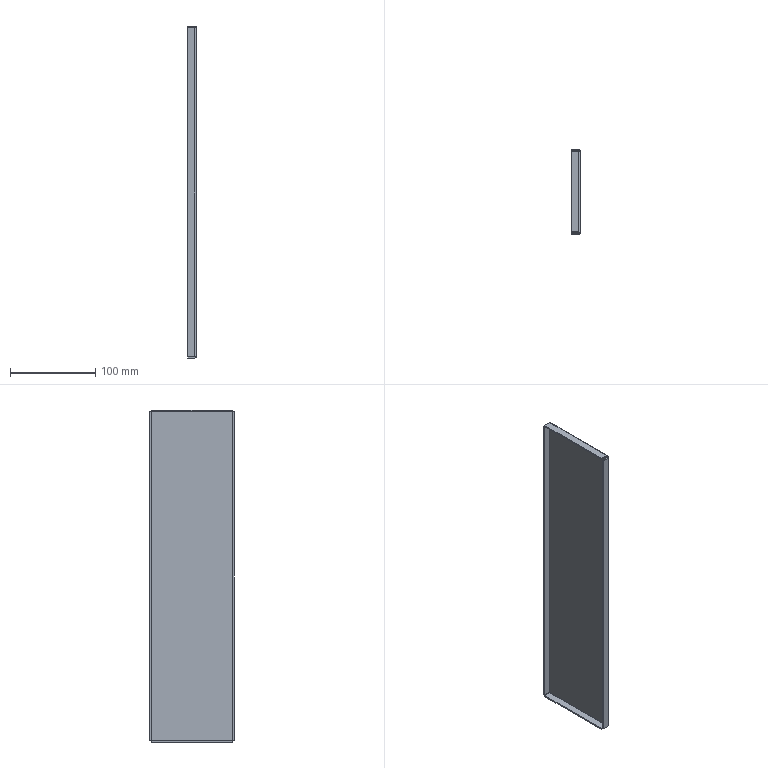Part | SolidWorks | 1 solid | 38 faces | box 10 x 99.001 x 390.001 mm | volume 69612 mm3 | plane 22 | spline 8 | cylinder 8 | commonest cylinder face diameters 0.2 x4 3.2 x4
STEP:
#1=CARTESIAN_POINT('',(-1.5,-47.9,-193.4));
#2=VERTEX_POINT('',#1);
#3=CARTESIAN_POINT('',(-1.5,47.9,-193.4));
#4=VERTEX_POINT('',#3);
#5=CARTESIAN_POINT('',(-1.5,-47.9,-193.4));
#6=DIRECTION('',(0.,1.,0.));
#7=VECTOR('',#6,1000.);
#8=LINE('',#5,#7);
#9=EDGE_CURVE('',#2,#4,#8,.T.);
#10=ORIENTED_EDGE('',*,*,#9,.F.);
#11=CARTESIAN_POINT('',(-1.5,-47.9,193.4));
#12=VERTEX_POINT('',#11);
#13=CARTESIAN_POINT('',(-1.5,-47.9,193.4));
#14=DIRECTION('',(0.,0.,-1.));
#15=VECTOR('',#14,1000.);
#16=LINE('',#13,#15);
#17=EDGE_CURVE('',#12,#2,#16,.T.);
#18=ORIENTED_EDGE('',*,*,#17,.F.);
#19=CARTESIAN_POINT('',(-1.5,47.9,193.4));
#20=VERTEX_POINT('',#19);
#21=CARTESIAN_POINT('',(-1.5,47.9,193.4));
#22=DIRECTION('',(0.,-1.,0.));
#23=VECTOR('',#22,1000.);
#24=LINE('',#21,#23);
#25=EDGE_CURVE('',#20,#12,#24,.T.);
#26=ORIENTED_EDGE('',*,*,#25,.F.);
#27=CARTESIAN_POINT('',(-1.5,47.9,-193.4));
#28=DIRECTION('',(0.,0.,1.));
#29=VECTOR('',#28,1000.);
#30=LINE('',#27,#29);
#31=EDGE_CURVE('',#4,#20,#30,.T.);
#32=ORIENTED_EDGE('',*,*,#31,.F.);
#33=EDGE_LOOP('',(#10,#18,#26,#32));
#34=FACE_OUTER_BOUND('',#33,.T.);
#35=CARTESIAN_POINT('',(-1.5,0.,0.));
#36=DIRECTION('',(1.,0.,0.));
#37=DIRECTION('',(0.,0.,-1.));
#38=AXIS2_PLACEMENT_3D('',#35,#36,#37);
#39=PLANE('',#38);
#40=ADVANCED_FACE('',(#34),#39,.F.);
#41=CARTESIAN_POINT('',(0.,-47.9,193.4));
#42=VERTEX_POINT('',#41);
#43=CARTESIAN_POINT('',(0.,-47.9,-193.4));
#44=VERTEX_POINT('',#43);
#45=CARTESIAN_POINT('',(0.,-47.9,193.4));
#46=DIRECTION('',(0.,0.,-1.));
#47=VECTOR('',#46,1000.);
#48=LINE('',#45,#47);
#49=EDGE_CURVE('',#42,#44,#48,.T.);
#50=ORIENTED_EDGE('',*,*,#49,.T.);
#51=CARTESIAN_POINT('',(0.,47.9,-193.4));
#52=VERTEX_POINT('',#51);
#53=CARTESIAN_POINT('',(0.,-47.9,-193.4));
#54=DIRECTION('',(0.,1.,0.));
#55=VECTOR('',#54,1000.);
#56=LINE('',#53,#55);
#57=EDGE_CURVE('',#44,#52,#56,.T.);
#58=ORIENTED_EDGE('',*,*,#57,.T.);
#59=CARTESIAN_POINT('',(0.,47.9,193.4));
#60=VERTEX_POINT('',#59);
#61=CARTESIAN_POINT('',(0.,47.9,-193.4));
#62=DIRECTION('',(0.,0.,1.));
#63=VECTOR('',#62,1000.);
#64=LINE('',#61,#63);
#65=EDGE_CURVE('',#52,#60,#64,.T.);
#66=ORIENTED_EDGE('',*,*,#65,.T.);
#67=CARTESIAN_POINT('',(0.,47.9,193.4));
#68=DIRECTION('',(0.,-1.,0.));
#69=VECTOR('',#68,1000.);
#70=LINE('',#67,#69);
#71=EDGE_CURVE('',#60,#42,#70,.T.);
#72=ORIENTED_EDGE('',*,*,#71,.T.);
#73=EDGE_LOOP('',(#50,#58,#66,#72));
#74=FACE_OUTER_BOUND('',#73,.T.);
#75=CARTESIAN_POINT('',(0.,0.,0.));
#76=DIRECTION('',(1.,0.,0.));
#77=DIRECTION('',(0.,0.,-1.));
#78=AXIS2_PLACEMENT_3D('',#75,#76,#77);
#79=PLANE('',#78);
#80=ADVANCED_FACE('',(#74),#79,.T.);
#81=CARTESIAN_POINT('',(-1.6,49.5,192.793));
#82=VERTEX_POINT('',#81);
#83=CARTESIAN_POINT('',(-1.6,48.,192.793));
#84=VERTEX_POINT('',#83);
#85=CARTESIAN_POINT('',(-1.6,48.,192.793));
#86=DIRECTION('',(0.,-1.,0.));
#87=VECTOR('',#86,1000.);
#88=LINE('',#85,#87);
#89=EDGE_CURVE('',#82,#84,#88,.T.);
#90=ORIENTED_EDGE('',*,*,#89,.T.);
#91=CARTESIAN_POINT('',(-1.5,47.9,193.4));
#92=CARTESIAN_POINT('',(-1.5,47.926,193.299));
#93=CARTESIAN_POINT('',(-1.511,47.952,193.198));
#94=CARTESIAN_POINT('',(-1.548,47.989,192.995));
#95=CARTESIAN_POINT('',(-1.574,48.,192.894));
#96=CARTESIAN_POINT('',(-1.6,48.,192.793));
#97=B_SPLINE_CURVE_WITH_KNOTS('',3,(#91,#92,#93,#94,#95,#96),.UNSPECIFIED.,.F.,.F.,(4,2,4),(0.,0.5,1.),.UNSPECIFIED.);
#98=EDGE_CURVE('',#20,#84,#97,.T.);
#99=ORIENTED_EDGE('',*,*,#98,.F.);
#100=CARTESIAN_POINT('',(-1.5,47.9,193.4));
#101=DIRECTION('',(1.,0.,0.));
#102=VECTOR('',#101,1000.);
#103=LINE('',#100,#102);
#104=EDGE_CURVE('',#20,#60,#103,.T.);
#105=ORIENTED_EDGE('',*,*,#104,.T.);
#106=CARTESIAN_POINT('',(0.,47.9,193.4));
#107=CARTESIAN_POINT('',(0.,48.112,193.349));
#108=CARTESIAN_POINT('',(-0.04048,48.315,193.3));
#109=CARTESIAN_POINT('',(-0.2012,48.705,193.198));
#110=CARTESIAN_POINT('',(-0.3186,48.881,193.148));
#111=CARTESIAN_POINT('',(-0.5418,49.105,193.071));
#112=CARTESIAN_POINT('',(-0.6225,49.171,193.046));
#113=CARTESIAN_POINT('',(-0.7959,49.287,192.996));
#114=CARTESIAN_POINT('',(-0.8897,49.338,192.97));
#115=CARTESIAN_POINT('',(-1.18,49.458,192.894));
#116=CARTESIAN_POINT('',(-1.388,49.5,192.844));
#117=CARTESIAN_POINT('',(-1.6,49.5,192.793));
#118=B_SPLINE_CURVE_WITH_KNOTS('',3,(#106,#107,#108,#109,#110,#111,#112,#113,#114,#115,#116,#117),.UNSPECIFIED.,.F.,.F.,(4,2,2,2,2,4),(0.,0.0006399,0.00128,0.0016,0.00192,0.00256),.UNSPECIFIED.);
#119=EDGE_CURVE('',#60,#82,#118,.T.);
#120=ORIENTED_EDGE('',*,*,#119,.T.);
#121=EDGE_LOOP('',(#90,#99,#105,#120));
#122=FACE_OUTER_BOUND('',#121,.T.);
#123=CARTESIAN_POINT('',(0.015,47.9,193.4));
#124=CARTESIAN_POINT('',(0.015,48.111,193.349));
#125=CARTESIAN_POINT('',(-0.02703,48.323,193.299));
#126=CARTESIAN_POINT('',(-0.1888,48.713,193.198));
#127=CARTESIAN_POINT('',(-0.3085,48.892,193.147));
#128=CARTESIAN_POINT('',(-0.6075,49.191,193.046));
#129=CARTESIAN_POINT('',(-0.7867,49.311,192.995));
#130=CARTESIAN_POINT('',(-1.177,49.473,192.894));
#131=CARTESIAN_POINT('',(-1.389,49.515,192.843));
#132=CARTESIAN_POINT('',(-1.6,49.515,192.793));
#133=CARTESIAN_POINT('',(0.,47.9,193.4));
#134=CARTESIAN_POINT('',(0.,48.109,193.349));
#135=CARTESIAN_POINT('',(-0.04164,48.319,193.299));
#136=CARTESIAN_POINT('',(-0.2019,48.706,193.198));
#137=CARTESIAN_POINT('',(-0.3205,48.883,193.147));
#138=CARTESIAN_POINT('',(-0.6167,49.179,193.046));
#139=CARTESIAN_POINT('',(-0.7942,49.298,192.995));
#140=CARTESIAN_POINT('',(-1.181,49.458,192.894));
#141=CARTESIAN_POINT('',(-1.391,49.5,192.843));
#142=CARTESIAN_POINT('',(-1.6,49.5,192.793));
#143=CARTESIAN_POINT('',(-1.5,47.9,193.4));
#144=CARTESIAN_POINT('',(-1.5,47.913,193.349));
#145=CARTESIAN_POINT('',(-1.503,47.926,193.299));
#146=CARTESIAN_POINT('',(-1.513,47.95,193.198));
#147=CARTESIAN_POINT('',(-1.52,47.961,193.147));
#148=CARTESIAN_POINT('',(-1.539,47.98,193.046));
#149=CARTESIAN_POINT('',(-1.55,47.987,192.995));
#150=CARTESIAN_POINT('',(-1.574,47.997,192.894));
#151=CARTESIAN_POINT('',(-1.587,48.,192.843));
#152=CARTESIAN_POINT('',(-1.6,48.,192.793));
#153=B_SPLINE_SURFACE_WITH_KNOTS('',1,3,((#123,#124,#125,#126,#127,#128,#129,#130,#131,#132),(#133,#134,#135,#136,#137,#138,#139,#140,#141,#142),(#143,#144,#145,#146,#147,#148,#149,#150,#151,#152)),.UNSPECIFIED.,.F.,.F.,.F.,(2,1,2),(4,2,2,2,4),(-0.01,0.,1.),(0.,0.25,0.5,0.75,1.),.UNSPECIFIED.);
#154=ADVANCED_FACE('',(#122),#153,.F.);
#155=CARTESIAN_POINT('',(-1.6,48.,-192.793));
#156=VERTEX_POINT('',#155);
#157=CARTESIAN_POINT('',(-1.6,48.,-192.793));
#158=CARTESIAN_POINT('',(-1.574,48.,-192.894));
#159=CARTESIAN_POINT('',(-1.548,47.989,-192.995));
#160=CARTESIAN_POINT('',(-1.511,47.952,-193.198));
#161=CARTESIAN_POINT('',(-1.5,47.926,-193.299));
#162=CARTESIAN_POINT('',(-1.5,47.9,-193.4));
#163=B_SPLINE_CURVE_WITH_KNOTS('',3,(#157,#158,#159,#160,#161,#162),.UNSPECIFIED.,.F.,.F.,(4,2,4),(0.,0.5,1.),.UNSPECIFIED.);
#164=EDGE_CURVE('',#156,#4,#163,.T.);
#165=ORIENTED_EDGE('',*,*,#164,.F.);
#166=CARTESIAN_POINT('',(-1.6,49.5,-192.793));
#167=VERTEX_POINT('',#166);
#168=CARTESIAN_POINT('',(-1.6,48.,-192.793));
#169=DIRECTION('',(0.,-1.,0.));
#170=VECTOR('',#169,1000.);
#171=LINE('',#168,#170);
#172=EDGE_CURVE('',#167,#156,#171,.T.);
#173=ORIENTED_EDGE('',*,*,#172,.F.);
#174=CARTESIAN_POINT('',(-1.6,49.5,-192.793));
#175=CARTESIAN_POINT('',(-1.388,49.5,-192.844));
#176=CARTESIAN_POINT('',(-1.185,49.46,-192.893));
#177=CARTESIAN_POINT('',(-0.7952,49.299,-192.995));
#178=CARTESIAN_POINT('',(-0.619,49.181,-193.045));
#179=CARTESIAN_POINT('',(-0.3953,48.958,-193.121));
#180=CARTESIAN_POINT('',(-0.329,48.878,-193.147));
#181=CARTESIAN_POINT('',(-0.2128,48.704,-193.197));
#182=CARTESIAN_POINT('',(-0.1625,48.61,-193.223));
#183=CARTESIAN_POINT('',(-0.04195,48.32,-193.299));
#184=CARTESIAN_POINT('',(0.,48.112,-193.349));
#185=CARTESIAN_POINT('',(0.,47.9,-193.4));
#186=B_SPLINE_CURVE_WITH_KNOTS('',3,(#174,#175,#176,#177,#178,#179,#180,#181,#182,#183,#184,#185),.UNSPECIFIED.,.F.,.F.,(4,2,2,2,2,4),(0.,0.0006399,0.00128,0.0016,0.00192,0.00256),.UNSPECIFIED.);
#187=EDGE_CURVE('',#167,#52,#186,.T.);
#188=ORIENTED_EDGE('',*,*,#187,.T.);
#189=CARTESIAN_POINT('',(-1.5,47.9,-193.4));
#190=DIRECTION('',(1.,0.,0.));
#191=VECTOR('',#190,1000.);
#192=LINE('',#189,#191);
#193=EDGE_CURVE('',#4,#52,#192,.T.);
#194=ORIENTED_EDGE('',*,*,#193,.F.);
#195=EDGE_LOOP('',(#165,#173,#188,#194));
#196=FACE_OUTER_BOUND('',#195,.T.);
#197=CARTESIAN_POINT('',(-1.6,49.515,-192.793));
#198=CARTESIAN_POINT('',(-1.389,49.515,-192.843));
#199=CARTESIAN_POINT('',(-1.177,49.473,-192.894));
#200=CARTESIAN_POINT('',(-0.7867,49.311,-192.995));
#201=CARTESIAN_POINT('',(-0.6075,49.191,-193.046));
#202=CARTESIAN_POINT('',(-0.3085,48.892,-193.147));
#203=CARTESIAN_POINT('',(-0.1888,48.713,-193.198));
#204=CARTESIAN_POINT('',(-0.02703,48.323,-193.299));
#205=CARTESIAN_POINT('',(0.015,48.111,-193.349));
#206=CARTESIAN_POINT('',(0.015,47.9,-193.4));
#207=CARTESIAN_POINT('',(-1.6,49.5,-192.793));
#208=CARTESIAN_POINT('',(-1.391,49.5,-192.843));
#209=CARTESIAN_POINT('',(-1.181,49.458,-192.894));
#210=CARTESIAN_POINT('',(-0.7942,49.298,-192.995));
#211=CARTESIAN_POINT('',(-0.6167,49.179,-193.046));
#212=CARTESIAN_POINT('',(-0.3205,48.883,-193.147));
#213=CARTESIAN_POINT('',(-0.2019,48.706,-193.198));
#214=CARTESIAN_POINT('',(-0.04164,48.319,-193.299));
#215=CARTESIAN_POINT('',(0.,48.109,-193.349));
#216=CARTESIAN_POINT('',(0.,47.9,-193.4));
#217=CARTESIAN_POINT('',(-1.6,48.,-192.793));
#218=CARTESIAN_POINT('',(-1.587,48.,-192.843));
#219=CARTESIAN_POINT('',(-1.574,47.997,-192.894));
#220=CARTESIAN_POINT('',(-1.55,47.987,-192.995));
#221=CARTESIAN_POINT('',(-1.539,47.98,-193.046));
#222=CARTESIAN_POINT('',(-1.52,47.961,-193.147));
#223=CARTESIAN_POINT('',(-1.513,47.95,-193.198));
#224=CARTESIAN_POINT('',(-1.503,47.926,-193.299));
#225=CARTESIAN_POINT('',(-1.5,47.913,-193.349));
#226=CARTESIAN_POINT('',(-1.5,47.9,-193.4));
#227=B_SPLINE_SURFACE_WITH_KNOTS('',1,3,((#197,#198,#199,#200,#201,#202,#203,#204,#205,#206),(#207,#208,#209,#210,#211,#212,#213,#214,#215,#216),(#217,#218,#219,#220,#221,#222,#223,#224,#225,#226)),.UNSPECIFIED.,.F.,.F.,.F.,(2,1,2),(4,2,2,2,4),(-0.01,0.,1.),(0.,0.25,0.5,0.75,1.),.UNSPECIFIED.);
#228=ADVANCED_FACE('',(#196),#227,.F.);
#229=ORIENTED_EDGE('',*,*,#65,.F.);
#230=ORIENTED_EDGE('',*,*,#187,.F.);
#231=CARTESIAN_POINT('',(-1.6,49.5,0.));
#232=DIRECTION('',(0.,0.,-1.));
#233=VECTOR('',#232,1000.);
#234=LINE('',#231,#233);
#235=EDGE_CURVE('',#82,#167,#234,.T.);
#236=ORIENTED_EDGE('',*,*,#235,.F.);
#237=ORIENTED_EDGE('',*,*,#119,.F.);
#238=EDGE_LOOP('',(#229,#230,#236,#237));
#239=FACE_OUTER_BOUND('',#238,.T.);
#240=CARTESIAN_POINT('',(-1.6,47.9,-193.4));
#241=DIRECTION('',(0.,0.,-1.));
#242=DIRECTION('',(0.,1.,0.));
#243=AXIS2_PLACEMENT_3D('',#240,#241,#242);
#244=CYLINDRICAL_SURFACE('',#243,1.6);
#245=ADVANCED_FACE('',(#239),#244,.T.);
#246=ORIENTED_EDGE('',*,*,#31,.T.);
#247=ORIENTED_EDGE('',*,*,#98,.T.);
#248=CARTESIAN_POINT('',(-1.6,48.,195.));
#249=DIRECTION('',(0.,0.,-1.));
#250=VECTOR('',#249,1000.);
#251=LINE('',#248,#250);
#252=EDGE_CURVE('',#84,#156,#251,.T.);
#253=ORIENTED_EDGE('',*,*,#252,.T.);
#254=ORIENTED_EDGE('',*,*,#164,.T.);
#255=EDGE_LOOP('',(#246,#247,#253,#254));
#256=FACE_OUTER_BOUND('',#255,.T.);
#257=CARTESIAN_POINT('',(-1.6,47.9,-193.4));
#258=DIRECTION('',(0.,0.,-1.));
#259=DIRECTION('',(0.,1.,0.));
#260=AXIS2_PLACEMENT_3D('',#257,#258,#259);
#261=CYLINDRICAL_SURFACE('',#260,0.1);
#262=ADVANCED_FACE('',(#256),#261,.F.);
#263=CARTESIAN_POINT('',(-10.,48.,192.793));
#264=VERTEX_POINT('',#263);
#265=CARTESIAN_POINT('',(-10.,49.5,192.793));
#266=VERTEX_POINT('',#265);
#267=CARTESIAN_POINT('',(-10.,49.5,192.793));
#268=DIRECTION('',(0.,1.,0.));
#269=VECTOR('',#268,1000.);
#270=LINE('',#267,#269);
#271=EDGE_CURVE('',#264,#266,#270,.T.);
#272=ORIENTED_EDGE('',*,*,#271,.F.);
#273=CARTESIAN_POINT('',(0.,48.,192.793));
#274=DIRECTION('',(-1.,0.,0.));
#275=VECTOR('',#274,1000.);
#276=LINE('',#273,#275);
#277=EDGE_CURVE('',#84,#264,#276,.T.);
#278=ORIENTED_EDGE('',*,*,#277,.F.);
#279=ORIENTED_EDGE('',*,*,#89,.F.);
#280=CARTESIAN_POINT('',(0.,49.5,192.793));
#281=DIRECTION('',(1.,0.,0.));
#282=VECTOR('',#281,1000.);
#283=LINE('',#280,#282);
#284=EDGE_CURVE('',#266,#82,#283,.T.);
#285=ORIENTED_EDGE('',*,*,#284,.F.);
#286=EDGE_LOOP('',(#272,#278,#279,#285));
#287=FACE_OUTER_BOUND('',#286,.T.);
#288=CARTESIAN_POINT('',(-1.5,48.,192.793));
#289=DIRECTION('',(0.,0.,1.));
#290=DIRECTION('',(1.,0.,0.));
#291=AXIS2_PLACEMENT_3D('',#288,#289,#290);
#292=PLANE('',#291);
#293=ADVANCED_FACE('',(#287),#292,.T.);
#294=CARTESIAN_POINT('',(-10.,49.5,-192.793));
#295=VERTEX_POINT('',#294);
#296=CARTESIAN_POINT('',(-1.5,49.5,-192.793));
#297=DIRECTION('',(1.,0.,0.));
#298=VECTOR('',#297,1000.);
#299=LINE('',#296,#298);
#300=EDGE_CURVE('',#295,#167,#299,.T.);
#301=ORIENTED_EDGE('',*,*,#300,.F.);
#302=CARTESIAN_POINT('',(-10.,49.5,-195.));
#303=DIRECTION('',(0.,0.,-1.));
#304=VECTOR('',#303,1000.);
#305=LINE('',#302,#304);
#306=EDGE_CURVE('',#266,#295,#305,.T.);
#307=ORIENTED_EDGE('',*,*,#306,.F.);
#308=ORIENTED_EDGE('',*,*,#284,.T.);
#309=ORIENTED_EDGE('',*,*,#235,.T.);
#310=EDGE_LOOP('',(#301,#307,#308,#309));
#311=FACE_OUTER_BOUND('',#310,.T.);
#312=CARTESIAN_POINT('',(0.,49.5,0.));
#313=DIRECTION('',(0.,1.,0.));
#314=DIRECTION('',(-1.,0.,0.));
#315=AXIS2_PLACEMENT_3D('',#312,#313,#314);
#316=PLANE('',#315);
#317=ADVANCED_FACE('',(#311),#316,.T.);
#318=CARTESIAN_POINT('',(-10.,48.,-192.793));
#319=VERTEX_POINT('',#318);
#320=CARTESIAN_POINT('',(-10.,48.,0.));
#321=DIRECTION('',(0.,0.,-1.));
#322=VECTOR('',#321,1000.);
#323=LINE('',#320,#322);
#324=EDGE_CURVE('',#264,#319,#323,.T.);
#325=ORIENTED_EDGE('',*,*,#324,.T.);
#326=CARTESIAN_POINT('',(-1.5,48.,-192.793));
#327=DIRECTION('',(-1.,0.,0.));
#328=VECTOR('',#327,1000.);
#329=LINE('',#326,#328);
#330=EDGE_CURVE('',#156,#319,#329,.T.);
#331=ORIENTED_EDGE('',*,*,#330,.F.);
#332=ORIENTED_EDGE('',*,*,#252,.F.);
#333=ORIENTED_EDGE('',*,*,#277,.T.);
#334=EDGE_LOOP('',(#325,#331,#332,#333));
#335=FACE_OUTER_BOUND('',#334,.T.);
#336=CARTESIAN_POINT('',(0.,48.,0.));
#337=DIRECTION('',(0.,1.,0.));
#338=DIRECTION('',(-1.,0.,0.));
#339=AXIS2_PLACEMENT_3D('',#336,#337,#338);
#340=PLANE('',#339);
#341=ADVANCED_FACE('',(#335),#340,.F.);
#342=CARTESIAN_POINT('',(-10.,48.,-192.793));
#343=DIRECTION('',(0.,1.,0.));
#344=VECTOR('',#343,1000.);
#345=LINE('',#342,#344);
#346=EDGE_CURVE('',#319,#295,#345,.T.);
#347=ORIENTED_EDGE('',*,*,#346,.F.);
#348=ORIENTED_EDGE('',*,*,#324,.F.);
#349=ORIENTED_EDGE('',*,*,#271,.T.);
#350=ORIENTED_EDGE('',*,*,#306,.T.);
#351=EDGE_LOOP('',(#347,#348,#349,#350));
#352=FACE_OUTER_BOUND('',#351,.T.);
#353=CARTESIAN_POINT('',(-10.,49.5,-195.));
#354=DIRECTION('',(-1.,0.,0.));
#355=DIRECTION('',(0.,-1.,0.));
#356=AXIS2_PLACEMENT_3D('',#353,#354,#355);
#357=PLANE('',#356);
#358=ADVANCED_FACE('',(#352),#357,.T.);
#359=ORIENTED_EDGE('',*,*,#330,.T.);
#360=ORIENTED_EDGE('',*,*,#346,.T.);
#361=ORIENTED_EDGE('',*,*,#300,.T.);
#362=ORIENTED_EDGE('',*,*,#172,.T.);
#363=EDGE_LOOP('',(#359,#360,#361,#362));
#364=FACE_OUTER_BOUND('',#363,.T.);
#365=CARTESIAN_POINT('',(-1.5,48.,-192.793));
#366=DIRECTION('',(0.,0.,1.));
#367=DIRECTION('',(1.,0.,0.));
#368=AXIS2_PLACEMENT_3D('',#365,#366,#367);
#369=PLANE('',#368);
#370=ADVANCED_FACE('',(#364),#369,.F.);
#371=CARTESIAN_POINT('',(-1.6,-47.293,195.));
#372=VERTEX_POINT('',#371);
#373=CARTESIAN_POINT('',(-1.6,-47.293,193.5));
#374=VERTEX_POINT('',#373);
#375=CARTESIAN_POINT('',(-1.6,-47.293,193.5));
#376=DIRECTION('',(0.,0.,-1.));
#377=VECTOR('',#376,1000.);
#378=LINE('',#375,#377);
#379=EDGE_CURVE('',#372,#374,#378,.T.);
#380=ORIENTED_EDGE('',*,*,#379,.T.);
#381=CARTESIAN_POINT('',(-1.5,-47.9,193.4));
#382=CARTESIAN_POINT('',(-1.5,-47.799,193.426));
#383=CARTESIAN_POINT('',(-1.511,-47.698,193.452));
#384=CARTESIAN_POINT('',(-1.548,-47.495,193.489));
#385=CARTESIAN_POINT('',(-1.574,-47.394,193.5));
#386=CARTESIAN_POINT('',(-1.6,-47.293,193.5));
#387=B_SPLINE_CURVE_WITH_KNOTS('',3,(#381,#382,#383,#384,#385,#386),.UNSPECIFIED.,.F.,.F.,(4,2,4),(0.,0.5,1.),.UNSPECIFIED.);
#388=EDGE_CURVE('',#12,#374,#387,.T.);
#389=ORIENTED_EDGE('',*,*,#388,.F.);
#390=CARTESIAN_POINT('',(-1.5,-47.9,193.4));
#391=DIRECTION('',(1.,0.,0.));
#392=VECTOR('',#391,1000.);
#393=LINE('',#390,#392);
#394=EDGE_CURVE('',#12,#42,#393,.T.);
#395=ORIENTED_EDGE('',*,*,#394,.T.);
#396=CARTESIAN_POINT('',(0.,-47.9,193.4));
#397=CARTESIAN_POINT('',(0.,-47.849,193.612));
#398=CARTESIAN_POINT('',(-0.04048,-47.8,193.815));
#399=CARTESIAN_POINT('',(-0.2012,-47.698,194.205));
#400=CARTESIAN_POINT('',(-0.3186,-47.648,194.381));
#401=CARTESIAN_POINT('',(-0.5418,-47.571,194.605));
#402=CARTESIAN_POINT('',(-0.6225,-47.546,194.671));
#403=CARTESIAN_POINT('',(-0.7959,-47.496,194.787));
#404=CARTESIAN_POINT('',(-0.8897,-47.47,194.838));
#405=CARTESIAN_POINT('',(-1.18,-47.394,194.958));
#406=CARTESIAN_POINT('',(-1.388,-47.344,195.));
#407=CARTESIAN_POINT('',(-1.6,-47.293,195.));
#408=B_SPLINE_CURVE_WITH_KNOTS('',3,(#396,#397,#398,#399,#400,#401,#402,#403,#404,#405,#406,#407),.UNSPECIFIED.,.F.,.F.,(4,2,2,2,2,4),(0.,0.0006399,0.00128,0.0016,0.00192,0.00256),.UNSPECIFIED.);
#409=EDGE_CURVE('',#42,#372,#408,.T.);
#410=ORIENTED_EDGE('',*,*,#409,.T.);
#411=EDGE_LOOP('',(#380,#389,#395,#410));
#412=FACE_OUTER_BOUND('',#411,.T.);
#413=CARTESIAN_POINT('',(0.015,-47.9,193.4));
#414=CARTESIAN_POINT('',(0.015,-47.849,193.611));
#415=CARTESIAN_POINT('',(-0.02703,-47.799,193.823));
#416=CARTESIAN_POINT('',(-0.1888,-47.698,194.213));
#417=CARTESIAN_POINT('',(-0.3085,-47.647,194.392));
#418=CARTESIAN_POINT('',(-0.6075,-47.546,194.691));
#419=CARTESIAN_POINT('',(-0.7867,-47.495,194.811));
#420=CARTESIAN_POINT('',(-1.177,-47.394,194.973));
#421=CARTESIAN_POINT('',(-1.389,-47.343,195.015));
#422=CARTESIAN_POINT('',(-1.6,-47.293,195.015));
#423=CARTESIAN_POINT('',(0.,-47.9,193.4));
#424=CARTESIAN_POINT('',(0.,-47.849,193.609));
#425=CARTESIAN_POINT('',(-0.04164,-47.799,193.819));
#426=CARTESIAN_POINT('',(-0.2019,-47.698,194.206));
#427=CARTESIAN_POINT('',(-0.3205,-47.647,194.383));
#428=CARTESIAN_POINT('',(-0.6167,-47.546,194.679));
#429=CARTESIAN_POINT('',(-0.7942,-47.495,194.798));
#430=CARTESIAN_POINT('',(-1.181,-47.394,194.958));
#431=CARTESIAN_POINT('',(-1.391,-47.343,195.));
#432=CARTESIAN_POINT('',(-1.6,-47.293,195.));
#433=CARTESIAN_POINT('',(-1.5,-47.9,193.4));
#434=CARTESIAN_POINT('',(-1.5,-47.849,193.413));
#435=CARTESIAN_POINT('',(-1.503,-47.799,193.426));
#436=CARTESIAN_POINT('',(-1.513,-47.698,193.45));
#437=CARTESIAN_POINT('',(-1.52,-47.647,193.461));
#438=CARTESIAN_POINT('',(-1.539,-47.546,193.48));
#439=CARTESIAN_POINT('',(-1.55,-47.495,193.487));
#440=CARTESIAN_POINT('',(-1.574,-47.394,193.497));
#441=CARTESIAN_POINT('',(-1.587,-47.343,193.5));
#442=CARTESIAN_POINT('',(-1.6,-47.293,193.5));
#443=B_SPLINE_SURFACE_WITH_KNOTS('',1,3,((#413,#414,#415,#416,#417,#418,#419,#420,#421,#422),(#423,#424,#425,#426,#427,#428,#429,#430,#431,#432),(#433,#434,#435,#436,#437,#438,#439,#440,#441,#442)),.UNSPECIFIED.,.F.,.F.,.F.,(2,1,2),(4,2,2,2,4),(-0.01,0.,1.),(0.,0.25,0.5,0.75,1.),.UNSPECIFIED.);
#444=ADVANCED_FACE('',(#412),#443,.F.);
#445=CARTESIAN_POINT('',(-1.6,47.293,193.5));
#446=VERTEX_POINT('',#445);
#447=CARTESIAN_POINT('',(-1.6,47.293,193.5));
#448=CARTESIAN_POINT('',(-1.574,47.394,193.5));
#449=CARTESIAN_POINT('',(-1.548,47.495,193.489));
#450=CARTESIAN_POINT('',(-1.511,47.698,193.452));
#451=CARTESIAN_POINT('',(-1.5,47.799,193.426));
#452=CARTESIAN_POINT('',(-1.5,47.9,193.4));
#453=B_SPLINE_CURVE_WITH_KNOTS('',3,(#447,#448,#449,#450,#451,#452),.UNSPECIFIED.,.F.,.F.,(4,2,4),(0.,0.5,1.),.UNSPECIFIED.);
#454=EDGE_CURVE('',#446,#20,#453,.T.);
#455=ORIENTED_EDGE('',*,*,#454,.F.);
#456=CARTESIAN_POINT('',(-1.6,47.293,195.));
#457=VERTEX_POINT('',#456);
#458=CARTESIAN_POINT('',(-1.6,47.293,193.5));
#459=DIRECTION('',(0.,0.,-1.));
#460=VECTOR('',#459,1000.);
#461=LINE('',#458,#460);
#462=EDGE_CURVE('',#457,#446,#461,.T.);
#463=ORIENTED_EDGE('',*,*,#462,.F.);
#464=CARTESIAN_POINT('',(-1.6,47.293,195.));
#465=CARTESIAN_POINT('',(-1.388,47.344,195.));
#466=CARTESIAN_POINT('',(-1.185,47.393,194.96));
#467=CARTESIAN_POINT('',(-0.7952,47.495,194.799));
#468=CARTESIAN_POINT('',(-0.619,47.545,194.681));
#469=CARTESIAN_POINT('',(-0.3953,47.621,194.458));
#470=CARTESIAN_POINT('',(-0.329,47.647,194.378));
#471=CARTESIAN_POINT('',(-0.2128,47.697,194.204));
#472=CARTESIAN_POINT('',(-0.1625,47.723,194.11));
#473=CARTESIAN_POINT('',(-0.04195,47.799,193.82));
#474=CARTESIAN_POINT('',(0.,47.849,193.612));
#475=CARTESIAN_POINT('',(0.,47.9,193.4));
#476=B_SPLINE_CURVE_WITH_KNOTS('',3,(#464,#465,#466,#467,#468,#469,#470,#471,#472,#473,#474,#475),.UNSPECIFIED.,.F.,.F.,(4,2,2,2,2,4),(0.,0.0006399,0.00128,0.0016,0.00192,0.00256),.UNSPECIFIED.);
#477=EDGE_CURVE('',#457,#60,#476,.T.);
#478=ORIENTED_EDGE('',*,*,#477,.T.);
#479=ORIENTED_EDGE('',*,*,#104,.F.);
#480=EDGE_LOOP('',(#455,#463,#478,#479));
#481=FACE_OUTER_BOUND('',#480,.T.);
#482=CARTESIAN_POINT('',(-1.6,47.293,195.015));
#483=CARTESIAN_POINT('',(-1.389,47.343,195.015));
#484=CARTESIAN_POINT('',(-1.177,47.394,194.973));
#485=CARTESIAN_POINT('',(-0.7867,47.495,194.811));
#486=CARTESIAN_POINT('',(-0.6075,47.546,194.691));
#487=CARTESIAN_POINT('',(-0.3085,47.647,194.392));
#488=CARTESIAN_POINT('',(-0.1888,47.698,194.213));
#489=CARTESIAN_POINT('',(-0.02703,47.799,193.823));
#490=CARTESIAN_POINT('',(0.015,47.849,193.611));
#491=CARTESIAN_POINT('',(0.015,47.9,193.4));
#492=CARTESIAN_POINT('',(-1.6,47.293,195.));
#493=CARTESIAN_POINT('',(-1.391,47.343,195.));
#494=CARTESIAN_POINT('',(-1.181,47.394,194.958));
#495=CARTESIAN_POINT('',(-0.7942,47.495,194.798));
#496=CARTESIAN_POINT('',(-0.6167,47.546,194.679));
#497=CARTESIAN_POINT('',(-0.3205,47.647,194.383));
#498=CARTESIAN_POINT('',(-0.2019,47.698,194.206));
#499=CARTESIAN_POINT('',(-0.04164,47.799,193.819));
#500=CARTESIAN_POINT('',(0.,47.849,193.609));
#501=CARTESIAN_POINT('',(0.,47.9,193.4));
#502=CARTESIAN_POINT('',(-1.6,47.293,193.5));
#503=CARTESIAN_POINT('',(-1.587,47.343,193.5));
#504=CARTESIAN_POINT('',(-1.574,47.394,193.497));
#505=CARTESIAN_POINT('',(-1.55,47.495,193.487));
#506=CARTESIAN_POINT('',(-1.539,47.546,193.48));
#507=CARTESIAN_POINT('',(-1.52,47.647,193.461));
#508=CARTESIAN_POINT('',(-1.513,47.698,193.45));
#509=CARTESIAN_POINT('',(-1.503,47.799,193.426));
#510=CARTESIAN_POINT('',(-1.5,47.849,193.413));
#511=CARTESIAN_POINT('',(-1.5,47.9,193.4));
#512=B_SPLINE_SURFACE_WITH_KNOTS('',1,3,((#482,#483,#484,#485,#486,#487,#488,#489,#490,#491),(#492,#493,#494,#495,#496,#497,#498,#499,#500,#501),(#502,#503,#504,#505,#506,#507,#508,#509,#510,#511)),.UNSPECIFIED.,.F.,.F.,.F.,(2,1,2),(4,2,2,2,4),(-0.01,0.,1.),(0.,0.25,0.5,0.75,1.),.UNSPECIFIED.);
#513=ADVANCED_FACE('',(#481),#512,.F.);
#514=ORIENTED_EDGE('',*,*,#71,.F.);
#515=ORIENTED_EDGE('',*,*,#477,.F.);
#516=CARTESIAN_POINT('',(-1.6,-49.5,195.));
#517=DIRECTION('',(0.,-1.,0.));
#518=VECTOR('',#517,1000.);
#519=LINE('',#516,#518);
#520=EDGE_CURVE('',#457,#372,#519,.T.);
#521=ORIENTED_EDGE('',*,*,#520,.T.);
#522=ORIENTED_EDGE('',*,*,#409,.F.);
#523=EDGE_LOOP('',(#514,#515,#521,#522));
#524=FACE_OUTER_BOUND('',#523,.T.);
#525=CARTESIAN_POINT('',(-1.6,47.9,193.4));
#526=DIRECTION('',(0.,1.,0.));
#527=DIRECTION('',(0.,0.,1.));
#528=AXIS2_PLACEMENT_3D('',#525,#526,#527);
#529=CYLINDRICAL_SURFACE('',#528,1.6);
#530=ADVANCED_FACE('',(#524),#529,.T.);
#531=ORIENTED_EDGE('',*,*,#25,.T.);
#532=ORIENTED_EDGE('',*,*,#388,.T.);
#533=CARTESIAN_POINT('',(-1.6,-49.5,193.5));
#534=DIRECTION('',(0.,1.,0.));
#535=VECTOR('',#534,1000.);
#536=LINE('',#533,#535);
#537=EDGE_CURVE('',#374,#446,#536,.T.);
#538=ORIENTED_EDGE('',*,*,#537,.T.);
#539=ORIENTED_EDGE('',*,*,#454,.T.);
#540=EDGE_LOOP('',(#531,#532,#538,#539));
#541=FACE_OUTER_BOUND('',#540,.T.);
#542=CARTESIAN_POINT('',(-1.6,47.9,193.4));
#543=DIRECTION('',(0.,1.,0.));
#544=DIRECTION('',(0.,0.,1.));
#545=AXIS2_PLACEMENT_3D('',#542,#543,#544);
#546=CYLINDRICAL_SURFACE('',#545,0.1);
#547=ADVANCED_FACE('',(#541),#546,.F.);
#548=CARTESIAN_POINT('',(-10.,-47.293,193.5));
#549=VERTEX_POINT('',#548);
#550=CARTESIAN_POINT('',(-10.,-47.293,195.));
#551=VERTEX_POINT('',#550);
#552=CARTESIAN_POINT('',(-10.,-47.293,195.));
#553=DIRECTION('',(0.,0.,1.));
#554=VECTOR('',#553,1000.);
#555=LINE('',#552,#554);
#556=EDGE_CURVE('',#549,#551,#555,.T.);
#557=ORIENTED_EDGE('',*,*,#556,.F.);
#558=CARTESIAN_POINT('',(0.,-47.293,193.5));
#559=DIRECTION('',(-1.,0.,0.));
#560=VECTOR('',#559,1000.);
#561=LINE('',#558,#560);
#562=EDGE_CURVE('',#374,#549,#561,.T.);
#563=ORIENTED_EDGE('',*,*,#562,.F.);
#564=ORIENTED_EDGE('',*,*,#379,.F.);
#565=CARTESIAN_POINT('',(-1.5,-47.293,195.));
#566=DIRECTION('',(-1.,0.,0.));
#567=VECTOR('',#566,1000.);
#568=LINE('',#565,#567);
#569=EDGE_CURVE('',#372,#551,#568,.T.);
#570=ORIENTED_EDGE('',*,*,#569,.T.);
#571=EDGE_LOOP('',(#557,#563,#564,#570));
#572=FACE_OUTER_BOUND('',#571,.T.);
#573=CARTESIAN_POINT('',(-1.5,-47.293,193.5));
#574=DIRECTION('',(0.,-1.,0.));
#575=DIRECTION('',(0.,0.,-1.));
#576=AXIS2_PLACEMENT_3D('',#573,#574,#575);
#577=PLANE('',#576);
#578=ADVANCED_FACE('',(#572),#577,.T.);
#579=ORIENTED_EDGE('',*,*,#520,.F.);
#580=CARTESIAN_POINT('',(-10.,47.293,195.));
#581=VERTEX_POINT('',#580);
#582=CARTESIAN_POINT('',(0.,47.293,195.));
#583=DIRECTION('',(-1.,0.,0.));
#584=VECTOR('',#583,1000.);
#585=LINE('',#582,#584);
#586=EDGE_CURVE('',#457,#581,#585,.T.);
#587=ORIENTED_EDGE('',*,*,#586,.T.);
#588=CARTESIAN_POINT('',(-10.,-49.5,195.));
#589=DIRECTION('',(0.,1.,0.));
#590=VECTOR('',#589,1000.);
#591=LINE('',#588,#590);
#592=EDGE_CURVE('',#551,#581,#591,.T.);
#593=ORIENTED_EDGE('',*,*,#592,.F.);
#594=ORIENTED_EDGE('',*,*,#569,.F.);
#595=EDGE_LOOP('',(#579,#587,#593,#594));
#596=FACE_OUTER_BOUND('',#595,.T.);
#597=CARTESIAN_POINT('',(0.,0.,195.));
#598=DIRECTION('',(0.,0.,-1.));
#599=DIRECTION('',(-1.,0.,0.));
#600=AXIS2_PLACEMENT_3D('',#597,#598,#599);
#601=PLANE('',#600);
#602=ADVANCED_FACE('',(#596),#601,.F.);
#603=CARTESIAN_POINT('',(-10.,47.293,193.5));
#604=VERTEX_POINT('',#603);
#605=CARTESIAN_POINT('',(-1.5,47.293,193.5));
#606=DIRECTION('',(-1.,0.,0.));
#607=VECTOR('',#606,1000.);
#608=LINE('',#605,#607);
#609=EDGE_CURVE('',#446,#604,#608,.T.);
#610=ORIENTED_EDGE('',*,*,#609,.F.);
#611=ORIENTED_EDGE('',*,*,#537,.F.);
#612=ORIENTED_EDGE('',*,*,#562,.T.);
#613=CARTESIAN_POINT('',(-10.,0.,193.5));
#614=DIRECTION('',(0.,1.,0.));
#615=VECTOR('',#614,1000.);
#616=LINE('',#613,#615);
#617=EDGE_CURVE('',#549,#604,#616,.T.);
#618=ORIENTED_EDGE('',*,*,#617,.T.);
#619=EDGE_LOOP('',(#610,#611,#612,#618));
#620=FACE_OUTER_BOUND('',#619,.T.);
#621=CARTESIAN_POINT('',(0.,0.,193.5));
#622=DIRECTION('',(0.,0.,-1.));
#623=DIRECTION('',(-1.,0.,0.));
#624=AXIS2_PLACEMENT_3D('',#621,#622,#623);
#625=PLANE('',#624);
#626=ADVANCED_FACE('',(#620),#625,.T.);
#627=CARTESIAN_POINT('',(-10.,47.293,193.5));
#628=DIRECTION('',(0.,0.,1.));
#629=VECTOR('',#628,1000.);
#630=LINE('',#627,#629);
#631=EDGE_CURVE('',#604,#581,#630,.T.);
#632=ORIENTED_EDGE('',*,*,#631,.F.);
#633=ORIENTED_EDGE('',*,*,#617,.F.);
#634=ORIENTED_EDGE('',*,*,#556,.T.);
#635=ORIENTED_EDGE('',*,*,#592,.T.);
#636=EDGE_LOOP('',(#632,#633,#634,#635));
#637=FACE_OUTER_BOUND('',#636,.T.);
#638=CARTESIAN_POINT('',(-10.,-49.5,195.));
#639=DIRECTION('',(-1.,0.,0.));
#640=DIRECTION('',(0.,0.,1.));
#641=AXIS2_PLACEMENT_3D('',#638,#639,#640);
#642=PLANE('',#641);
#643=ADVANCED_FACE('',(#637),#642,.T.);
#644=ORIENTED_EDGE('',*,*,#609,.T.);
#645=ORIENTED_EDGE('',*,*,#631,.T.);
#646=ORIENTED_EDGE('',*,*,#586,.F.);
#647=ORIENTED_EDGE('',*,*,#462,.T.);
#648=EDGE_LOOP('',(#644,#645,#646,#647));
#649=FACE_OUTER_BOUND('',#648,.T.);
#650=CARTESIAN_POINT('',(-1.5,47.293,193.5));
#651=DIRECTION('',(0.,-1.,0.));
#652=DIRECTION('',(0.,0.,-1.));
#653=AXIS2_PLACEMENT_3D('',#650,#651,#652);
#654=PLANE('',#653);
#655=ADVANCED_FACE('',(#649),#654,.F.);
#656=CARTESIAN_POINT('',(-1.6,-49.5,-192.793));
#657=VERTEX_POINT('',#656);
#658=CARTESIAN_POINT('',(-1.6,-48.,-192.793));
#659=VERTEX_POINT('',#658);
#660=CARTESIAN_POINT('',(-1.6,-48.,-192.793));
#661=DIRECTION('',(0.,1.,0.));
#662=VECTOR('',#661,1000.);
#663=LINE('',#660,#662);
#664=EDGE_CURVE('',#657,#659,#663,.T.);
#665=ORIENTED_EDGE('',*,*,#664,.T.);
#666=CARTESIAN_POINT('',(-1.5,-47.9,-193.4));
#667=CARTESIAN_POINT('',(-1.5,-47.926,-193.299));
#668=CARTESIAN_POINT('',(-1.511,-47.952,-193.198));
#669=CARTESIAN_POINT('',(-1.548,-47.989,-192.995));
#670=CARTESIAN_POINT('',(-1.574,-48.,-192.894));
#671=CARTESIAN_POINT('',(-1.6,-48.,-192.793));
#672=B_SPLINE_CURVE_WITH_KNOTS('',3,(#666,#667,#668,#669,#670,#671),.UNSPECIFIED.,.F.,.F.,(4,2,4),(0.,0.5,1.),.UNSPECIFIED.);
#673=EDGE_CURVE('',#2,#659,#672,.T.);
#674=ORIENTED_EDGE('',*,*,#673,.F.);
#675=CARTESIAN_POINT('',(-1.5,-47.9,-193.4));
#676=DIRECTION('',(1.,0.,0.));
#677=VECTOR('',#676,1000.);
#678=LINE('',#675,#677);
#679=EDGE_CURVE('',#2,#44,#678,.T.);
#680=ORIENTED_EDGE('',*,*,#679,.T.);
#681=CARTESIAN_POINT('',(0.,-47.9,-193.4));
#682=CARTESIAN_POINT('',(0.,-48.112,-193.349));
#683=CARTESIAN_POINT('',(-0.04048,-48.315,-193.3));
#684=CARTESIAN_POINT('',(-0.2012,-48.705,-193.198));
#685=CARTESIAN_POINT('',(-0.3186,-48.881,-193.148));
#686=CARTESIAN_POINT('',(-0.5418,-49.105,-193.071));
#687=CARTESIAN_POINT('',(-0.6225,-49.171,-193.046));
#688=CARTESIAN_POINT('',(-0.7959,-49.287,-192.996));
#689=CARTESIAN_POINT('',(-0.8897,-49.338,-192.97));
#690=CARTESIAN_POINT('',(-1.18,-49.458,-192.894));
#691=CARTESIAN_POINT('',(-1.388,-49.5,-192.844));
#692=CARTESIAN_POINT('',(-1.6,-49.5,-192.793));
#693=B_SPLINE_CURVE_WITH_KNOTS('',3,(#681,#682,#683,#684,#685,#686,#687,#688,#689,#690,#691,#692),.UNSPECIFIED.,.F.,.F.,(4,2,2,2,2,4),(0.,0.0006399,0.00128,0.0016,0.00192,0.00256),.UNSPECIFIED.);
#694=EDGE_CURVE('',#44,#657,#693,.T.);
#695=ORIENTED_EDGE('',*,*,#694,.T.);
#696=EDGE_LOOP('',(#665,#674,#680,#695));
#697=FACE_OUTER_BOUND('',#696,.T.);
#698=CARTESIAN_POINT('',(0.015,-47.9,-193.4));
#699=CARTESIAN_POINT('',(0.015,-48.111,-193.349));
#700=CARTESIAN_POINT('',(-0.02703,-48.323,-193.299));
#701=CARTESIAN_POINT('',(-0.1888,-48.713,-193.198));
#702=CARTESIAN_POINT('',(-0.3085,-48.892,-193.147));
#703=CARTESIAN_POINT('',(-0.6075,-49.191,-193.046));
#704=CARTESIAN_POINT('',(-0.7867,-49.311,-192.995));
#705=CARTESIAN_POINT('',(-1.177,-49.473,-192.894));
#706=CARTESIAN_POINT('',(-1.389,-49.515,-192.843));
#707=CARTESIAN_POINT('',(-1.6,-49.515,-192.793));
#708=CARTESIAN_POINT('',(0.,-47.9,-193.4));
#709=CARTESIAN_POINT('',(0.,-48.109,-193.349));
#710=CARTESIAN_POINT('',(-0.04164,-48.319,-193.299));
#711=CARTESIAN_POINT('',(-0.2019,-48.706,-193.198));
#712=CARTESIAN_POINT('',(-0.3205,-48.883,-193.147));
#713=CARTESIAN_POINT('',(-0.6167,-49.179,-193.046));
#714=CARTESIAN_POINT('',(-0.7942,-49.298,-192.995));
#715=CARTESIAN_POINT('',(-1.181,-49.458,-192.894));
#716=CARTESIAN_POINT('',(-1.391,-49.5,-192.843));
#717=CARTESIAN_POINT('',(-1.6,-49.5,-192.793));
#718=CARTESIAN_POINT('',(-1.5,-47.9,-193.4));
#719=CARTESIAN_POINT('',(-1.5,-47.913,-193.349));
#720=CARTESIAN_POINT('',(-1.503,-47.926,-193.299));
#721=CARTESIAN_POINT('',(-1.513,-47.95,-193.198));
#722=CARTESIAN_POINT('',(-1.52,-47.961,-193.147));
#723=CARTESIAN_POINT('',(-1.539,-47.98,-193.046));
#724=CARTESIAN_POINT('',(-1.55,-47.987,-192.995));
#725=CARTESIAN_POINT('',(-1.574,-47.997,-192.894));
#726=CARTESIAN_POINT('',(-1.587,-48.,-192.843));
#727=CARTESIAN_POINT('',(-1.6,-48.,-192.793));
#728=B_SPLINE_SURFACE_WITH_KNOTS('',1,3,((#698,#699,#700,#701,#702,#703,#704,#705,#706,#707),(#708,#709,#710,#711,#712,#713,#714,#715,#716,#717),(#718,#719,#720,#721,#722,#723,#724,#725,#726,#727)),.UNSPECIFIED.,.F.,.F.,.F.,(2,1,2),(4,2,2,2,4),(-0.01,0.,1.),(0.,0.25,0.5,0.75,1.),.UNSPECIFIED.);
#729=ADVANCED_FACE('',(#697),#728,.F.);
#730=CARTESIAN_POINT('',(-1.6,-48.,192.793));
#731=VERTEX_POINT('',#730);
#732=CARTESIAN_POINT('',(-1.6,-48.,192.793));
#733=CARTESIAN_POINT('',(-1.574,-48.,192.894));
#734=CARTESIAN_POINT('',(-1.548,-47.989,192.995));
#735=CARTESIAN_POINT('',(-1.511,-47.952,193.198));
#736=CARTESIAN_POINT('',(-1.5,-47.926,193.299));
#737=CARTESIAN_POINT('',(-1.5,-47.9,193.4));
#738=B_SPLINE_CURVE_WITH_KNOTS('',3,(#732,#733,#734,#735,#736,#737),.UNSPECIFIED.,.F.,.F.,(4,2,4),(0.,0.5,1.),.UNSPECIFIED.);
#739=EDGE_CURVE('',#731,#12,#738,.T.);
#740=ORIENTED_EDGE('',*,*,#739,.F.);
#741=CARTESIAN_POINT('',(-1.6,-49.5,192.793));
#742=VERTEX_POINT('',#741);
#743=CARTESIAN_POINT('',(-1.6,-48.,192.793));
#744=DIRECTION('',(0.,1.,0.));
#745=VECTOR('',#744,1000.);
#746=LINE('',#743,#745);
#747=EDGE_CURVE('',#742,#731,#746,.T.);
#748=ORIENTED_EDGE('',*,*,#747,.F.);
#749=CARTESIAN_POINT('',(-1.6,-49.5,192.793));
#750=CARTESIAN_POINT('',(-1.388,-49.5,192.844));
#751=CARTESIAN_POINT('',(-1.185,-49.46,192.893));
#752=CARTESIAN_POINT('',(-0.7952,-49.299,192.995));
#753=CARTESIAN_POINT('',(-0.619,-49.181,193.045));
#754=CARTESIAN_POINT('',(-0.3953,-48.958,193.121));
#755=CARTESIAN_POINT('',(-0.329,-48.878,193.147));
#756=CARTESIAN_POINT('',(-0.2128,-48.704,193.197));
#757=CARTESIAN_POINT('',(-0.1625,-48.61,193.223));
#758=CARTESIAN_POINT('',(-0.04195,-48.32,193.299));
#759=CARTESIAN_POINT('',(0.,-48.112,193.349));
#760=CARTESIAN_POINT('',(0.,-47.9,193.4));
#761=B_SPLINE_CURVE_WITH_KNOTS('',3,(#749,#750,#751,#752,#753,#754,#755,#756,#757,#758,#759,#760),.UNSPECIFIED.,.F.,.F.,(4,2,2,2,2,4),(0.,0.0006399,0.00128,0.0016,0.00192,0.00256),.UNSPECIFIED.);
#762=EDGE_CURVE('',#742,#42,#761,.T.);
#763=ORIENTED_EDGE('',*,*,#762,.T.);
#764=ORIENTED_EDGE('',*,*,#394,.F.);
#765=EDGE_LOOP('',(#740,#748,#763,#764));
#766=FACE_OUTER_BOUND('',#765,.T.);
#767=CARTESIAN_POINT('',(-1.6,-49.515,192.793));
#768=CARTESIAN_POINT('',(-1.389,-49.515,192.843));
#769=CARTESIAN_POINT('',(-1.177,-49.473,192.894));
#770=CARTESIAN_POINT('',(-0.7867,-49.311,192.995));
#771=CARTESIAN_POINT('',(-0.6075,-49.191,193.046));
#772=CARTESIAN_POINT('',(-0.3085,-48.892,193.147));
#773=CARTESIAN_POINT('',(-0.1888,-48.713,193.198));
#774=CARTESIAN_POINT('',(-0.02703,-48.323,193.299));
#775=CARTESIAN_POINT('',(0.015,-48.111,193.349));
#776=CARTESIAN_POINT('',(0.015,-47.9,193.4));
#777=CARTESIAN_POINT('',(-1.6,-49.5,192.793));
#778=CARTESIAN_POINT('',(-1.391,-49.5,192.843));
#779=CARTESIAN_POINT('',(-1.181,-49.458,192.894));
#780=CARTESIAN_POINT('',(-0.7942,-49.298,192.995));
#781=CARTESIAN_POINT('',(-0.6167,-49.179,193.046));
#782=CARTESIAN_POINT('',(-0.3205,-48.883,193.147));
#783=CARTESIAN_POINT('',(-0.2019,-48.706,193.198));
#784=CARTESIAN_POINT('',(-0.04164,-48.319,193.299));
#785=CARTESIAN_POINT('',(0.,-48.109,193.349));
#786=CARTESIAN_POINT('',(0.,-47.9,193.4));
#787=CARTESIAN_POINT('',(-1.6,-48.,192.793));
#788=CARTESIAN_POINT('',(-1.587,-48.,192.843));
#789=CARTESIAN_POINT('',(-1.574,-47.997,192.894));
#790=CARTESIAN_POINT('',(-1.55,-47.987,192.995));
#791=CARTESIAN_POINT('',(-1.539,-47.98,193.046));
#792=CARTESIAN_POINT('',(-1.52,-47.961,193.147));
#793=CARTESIAN_POINT('',(-1.513,-47.95,193.198));
#794=CARTESIAN_POINT('',(-1.503,-47.926,193.299));
#795=CARTESIAN_POINT('',(-1.5,-47.913,193.349));
#796=CARTESIAN_POINT('',(-1.5,-47.9,193.4));
#797=B_SPLINE_SURFACE_WITH_KNOTS('',1,3,((#767,#768,#769,#770,#771,#772,#773,#774,#775,#776),(#777,#778,#779,#780,#781,#782,#783,#784,#785,#786),(#787,#788,#789,#790,#791,#792,#793,#794,#795,#796)),.UNSPECIFIED.,.F.,.F.,.F.,(2,1,2),(4,2,2,2,4),(-0.01,0.,1.),(0.,0.25,0.5,0.75,1.),.UNSPECIFIED.);
#798=ADVANCED_FACE('',(#766),#797,.F.);
#799=ORIENTED_EDGE('',*,*,#49,.F.);
#800=ORIENTED_EDGE('',*,*,#762,.F.);
#801=CARTESIAN_POINT('',(-1.6,-49.5,-195.));
#802=DIRECTION('',(0.,0.,-1.));
#803=VECTOR('',#802,1000.);
#804=LINE('',#801,#803);
#805=EDGE_CURVE('',#742,#657,#804,.T.);
#806=ORIENTED_EDGE('',*,*,#805,.T.);
#807=ORIENTED_EDGE('',*,*,#694,.F.);
#808=EDGE_LOOP('',(#799,#800,#806,#807));
#809=FACE_OUTER_BOUND('',#808,.T.);
#810=CARTESIAN_POINT('',(-1.6,-47.9,193.4));
#811=DIRECTION('',(0.,0.,1.));
#812=DIRECTION('',(0.,-1.,0.));
#813=AXIS2_PLACEMENT_3D('',#810,#811,#812);
#814=CYLINDRICAL_SURFACE('',#813,1.6);
#815=ADVANCED_FACE('',(#809),#814,.T.);
#816=ORIENTED_EDGE('',*,*,#17,.T.);
#817=ORIENTED_EDGE('',*,*,#673,.T.);
#818=CARTESIAN_POINT('',(-1.6,-48.,-195.));
#819=DIRECTION('',(0.,0.,1.));
#820=VECTOR('',#819,1000.);
#821=LINE('',#818,#820);
#822=EDGE_CURVE('',#659,#731,#821,.T.);
#823=ORIENTED_EDGE('',*,*,#822,.T.);
#824=ORIENTED_EDGE('',*,*,#739,.T.);
#825=EDGE_LOOP('',(#816,#817,#823,#824));
#826=FACE_OUTER_BOUND('',#825,.T.);
#827=CARTESIAN_POINT('',(-1.6,-47.9,193.4));
#828=DIRECTION('',(0.,0.,1.));
#829=DIRECTION('',(0.,-1.,0.));
#830=AXIS2_PLACEMENT_3D('',#827,#828,#829);
#831=CYLINDRICAL_SURFACE('',#830,0.1);
#832=ADVANCED_FACE('',(#826),#831,.F.);
#833=CARTESIAN_POINT('',(-10.,-48.,-192.793));
#834=VERTEX_POINT('',#833);
#835=CARTESIAN_POINT('',(-10.,-49.5,-192.793));
#836=VERTEX_POINT('',#835);
#837=CARTESIAN_POINT('',(-10.,-49.5,-192.793));
#838=DIRECTION('',(0.,-1.,0.));
#839=VECTOR('',#838,1000.);
#840=LINE('',#837,#839);
#841=EDGE_CURVE('',#834,#836,#840,.T.);
#842=ORIENTED_EDGE('',*,*,#841,.F.);
#843=CARTESIAN_POINT('',(0.,-48.,-192.793));
#844=DIRECTION('',(-1.,0.,0.));
#845=VECTOR('',#844,1000.);
#846=LINE('',#843,#845);
#847=EDGE_CURVE('',#659,#834,#846,.T.);
#848=ORIENTED_EDGE('',*,*,#847,.F.);
#849=ORIENTED_EDGE('',*,*,#664,.F.);
#850=CARTESIAN_POINT('',(-1.5,-49.5,-192.793));
#851=DIRECTION('',(-1.,0.,0.));
#852=VECTOR('',#851,1000.);
#853=LINE('',#850,#852);
#854=EDGE_CURVE('',#657,#836,#853,.T.);
#855=ORIENTED_EDGE('',*,*,#854,.T.);
#856=EDGE_LOOP('',(#842,#848,#849,#855));
#857=FACE_OUTER_BOUND('',#856,.T.);
#858=CARTESIAN_POINT('',(-1.5,-48.,-192.793));
#859=DIRECTION('',(0.,0.,-1.));
#860=DIRECTION('',(-1.,0.,0.));
#861=AXIS2_PLACEMENT_3D('',#858,#859,#860);
#862=PLANE('',#861);
#863=ADVANCED_FACE('',(#857),#862,.T.);
#864=ORIENTED_EDGE('',*,*,#805,.F.);
#865=CARTESIAN_POINT('',(-10.,-49.5,192.793));
#866=VERTEX_POINT('',#865);
#867=CARTESIAN_POINT('',(0.,-49.5,192.793));
#868=DIRECTION('',(-1.,0.,0.));
#869=VECTOR('',#868,1000.);
#870=LINE('',#867,#869);
#871=EDGE_CURVE('',#742,#866,#870,.T.);
#872=ORIENTED_EDGE('',*,*,#871,.T.);
#873=CARTESIAN_POINT('',(-10.,-49.5,-195.));
#874=DIRECTION('',(0.,0.,1.));
#875=VECTOR('',#874,1000.);
#876=LINE('',#873,#875);
#877=EDGE_CURVE('',#836,#866,#876,.T.);
#878=ORIENTED_EDGE('',*,*,#877,.F.);
#879=ORIENTED_EDGE('',*,*,#854,.F.);
#880=EDGE_LOOP('',(#864,#872,#878,#879));
#881=FACE_OUTER_BOUND('',#880,.T.);
#882=CARTESIAN_POINT('',(0.,-49.5,0.));
#883=DIRECTION('',(0.,1.,0.));
#884=DIRECTION('',(-1.,0.,0.));
#885=AXIS2_PLACEMENT_3D('',#882,#883,#884);
#886=PLANE('',#885);
#887=ADVANCED_FACE('',(#881),#886,.F.);
#888=CARTESIAN_POINT('',(-10.,-48.,192.793));
#889=VERTEX_POINT('',#888);
#890=CARTESIAN_POINT('',(-1.5,-48.,192.793));
#891=DIRECTION('',(-1.,0.,0.));
#892=VECTOR('',#891,1000.);
#893=LINE('',#890,#892);
#894=EDGE_CURVE('',#731,#889,#893,.T.);
#895=ORIENTED_EDGE('',*,*,#894,.F.);
#896=ORIENTED_EDGE('',*,*,#822,.F.);
#897=ORIENTED_EDGE('',*,*,#847,.T.);
#898=CARTESIAN_POINT('',(-10.,-48.,0.));
#899=DIRECTION('',(0.,0.,1.));
#900=VECTOR('',#899,1000.);
#901=LINE('',#898,#900);
#902=EDGE_CURVE('',#834,#889,#901,.T.);
#903=ORIENTED_EDGE('',*,*,#902,.T.);
#904=EDGE_LOOP('',(#895,#896,#897,#903));
#905=FACE_OUTER_BOUND('',#904,.T.);
#906=CARTESIAN_POINT('',(0.,-48.,0.));
#907=DIRECTION('',(0.,1.,0.));
#908=DIRECTION('',(-1.,0.,0.));
#909=AXIS2_PLACEMENT_3D('',#906,#907,#908);
#910=PLANE('',#909);
#911=ADVANCED_FACE('',(#905),#910,.T.);
#912=CARTESIAN_POINT('',(-10.,-48.,192.793));
#913=DIRECTION('',(0.,-1.,0.));
#914=VECTOR('',#913,1000.);
#915=LINE('',#912,#914);
#916=EDGE_CURVE('',#889,#866,#915,.T.);
#917=ORIENTED_EDGE('',*,*,#916,.F.);
#918=ORIENTED_EDGE('',*,*,#902,.F.);
#919=ORIENTED_EDGE('',*,*,#841,.T.);
#920=ORIENTED_EDGE('',*,*,#877,.T.);
#921=EDGE_LOOP('',(#917,#918,#919,#920));
#922=FACE_OUTER_BOUND('',#921,.T.);
#923=CARTESIAN_POINT('',(-10.,-49.5,-195.));
#924=DIRECTION('',(-1.,0.,0.));
#925=DIRECTION('',(0.,-1.,0.));
#926=AXIS2_PLACEMENT_3D('',#923,#924,#925);
#927=PLANE('',#926);
#928=ADVANCED_FACE('',(#922),#927,.T.);
#929=ORIENTED_EDGE('',*,*,#894,.T.);
#930=ORIENTED_EDGE('',*,*,#916,.T.);
#931=ORIENTED_EDGE('',*,*,#871,.F.);
#932=ORIENTED_EDGE('',*,*,#747,.T.);
#933=EDGE_LOOP('',(#929,#930,#931,#932));
#934=FACE_OUTER_BOUND('',#933,.T.);
#935=CARTESIAN_POINT('',(-1.5,-48.,192.793));
#936=DIRECTION('',(0.,0.,-1.));
#937=DIRECTION('',(-1.,0.,0.));
#938=AXIS2_PLACEMENT_3D('',#935,#936,#937);
#939=PLANE('',#938);
#940=ADVANCED_FACE('',(#934),#939,.F.);
#941=CARTESIAN_POINT('',(-1.6,47.293,-195.));
#942=VERTEX_POINT('',#941);
#943=CARTESIAN_POINT('',(-1.6,47.293,-193.5));
#944=VERTEX_POINT('',#943);
#945=CARTESIAN_POINT('',(-1.6,47.293,-193.5));
#946=DIRECTION('',(0.,0.,1.));
#947=VECTOR('',#946,1000.);
#948=LINE('',#945,#947);
#949=EDGE_CURVE('',#942,#944,#948,.T.);
#950=ORIENTED_EDGE('',*,*,#949,.T.);
#951=CARTESIAN_POINT('',(-1.5,47.9,-193.4));
#952=CARTESIAN_POINT('',(-1.5,47.799,-193.426));
#953=CARTESIAN_POINT('',(-1.511,47.698,-193.452));
#954=CARTESIAN_POINT('',(-1.548,47.495,-193.489));
#955=CARTESIAN_POINT('',(-1.574,47.394,-193.5));
#956=CARTESIAN_POINT('',(-1.6,47.293,-193.5));
#957=B_SPLINE_CURVE_WITH_KNOTS('',3,(#951,#952,#953,#954,#955,#956),.UNSPECIFIED.,.F.,.F.,(4,2,4),(0.,0.5,1.),.UNSPECIFIED.);
#958=EDGE_CURVE('',#4,#944,#957,.T.);
#959=ORIENTED_EDGE('',*,*,#958,.F.);
#960=ORIENTED_EDGE('',*,*,#193,.T.);
#961=CARTESIAN_POINT('',(0.,47.9,-193.4));
#962=CARTESIAN_POINT('',(0.,47.849,-193.612));
#963=CARTESIAN_POINT('',(-0.04048,47.8,-193.815));
#964=CARTESIAN_POINT('',(-0.2012,47.698,-194.205));
#965=CARTESIAN_POINT('',(-0.3186,47.648,-194.381));
#966=CARTESIAN_POINT('',(-0.5418,47.571,-194.605));
#967=CARTESIAN_POINT('',(-0.6225,47.546,-194.671));
#968=CARTESIAN_POINT('',(-0.7959,47.496,-194.787));
#969=CARTESIAN_POINT('',(-0.8897,47.47,-194.838));
#970=CARTESIAN_POINT('',(-1.18,47.394,-194.958));
#971=CARTESIAN_POINT('',(-1.388,47.344,-195.));
#972=CARTESIAN_POINT('',(-1.6,47.293,-195.));
#973=B_SPLINE_CURVE_WITH_KNOTS('',3,(#961,#962,#963,#964,#965,#966,#967,#968,#969,#970,#971,#972),.UNSPECIFIED.,.F.,.F.,(4,2,2,2,2,4),(0.,0.0006399,0.00128,0.0016,0.00192,0.00256),.UNSPECIFIED.);
#974=EDGE_CURVE('',#52,#942,#973,.T.);
#975=ORIENTED_EDGE('',*,*,#974,.T.);
#976=EDGE_LOOP('',(#950,#959,#960,#975));
#977=FACE_OUTER_BOUND('',#976,.T.);
#978=CARTESIAN_POINT('',(0.015,47.9,-193.4));
#979=CARTESIAN_POINT('',(0.015,47.849,-193.611));
#980=CARTESIAN_POINT('',(-0.02703,47.799,-193.823));
#981=CARTESIAN_POINT('',(-0.1888,47.698,-194.213));
#982=CARTESIAN_POINT('',(-0.3085,47.647,-194.392));
#983=CARTESIAN_POINT('',(-0.6075,47.546,-194.691));
#984=CARTESIAN_POINT('',(-0.7867,47.495,-194.811));
#985=CARTESIAN_POINT('',(-1.177,47.394,-194.973));
#986=CARTESIAN_POINT('',(-1.389,47.343,-195.015));
#987=CARTESIAN_POINT('',(-1.6,47.293,-195.015));
#988=CARTESIAN_POINT('',(0.,47.9,-193.4));
#989=CARTESIAN_POINT('',(0.,47.849,-193.609));
#990=CARTESIAN_POINT('',(-0.04164,47.799,-193.819));
#991=CARTESIAN_POINT('',(-0.2019,47.698,-194.206));
#992=CARTESIAN_POINT('',(-0.3205,47.647,-194.383));
#993=CARTESIAN_POINT('',(-0.6167,47.546,-194.679));
#994=CARTESIAN_POINT('',(-0.7942,47.495,-194.798));
#995=CARTESIAN_POINT('',(-1.181,47.394,-194.958));
#996=CARTESIAN_POINT('',(-1.391,47.343,-195.));
#997=CARTESIAN_POINT('',(-1.6,47.293,-195.));
#998=CARTESIAN_POINT('',(-1.5,47.9,-193.4));
#999=CARTESIAN_POINT('',(-1.5,47.849,-193.413));
#1000=CARTESIAN_POINT('',(-1.503,47.799,-193.426));
#1001=CARTESIAN_POINT('',(-1.513,47.698,-193.45));
#1002=CARTESIAN_POINT('',(-1.52,47.647,-193.461));
#1003=CARTESIAN_POINT('',(-1.539,47.546,-193.48));
#1004=CARTESIAN_POINT('',(-1.55,47.495,-193.487));
#1005=CARTESIAN_POINT('',(-1.574,47.394,-193.497));
#1006=CARTESIAN_POINT('',(-1.587,47.343,-193.5));
#1007=CARTESIAN_POINT('',(-1.6,47.293,-193.5));
#1008=B_SPLINE_SURFACE_WITH_KNOTS('',1,3,((#978,#979,#980,#981,#982,#983,#984,#985,#986,#987),(#988,#989,#990,#991,#992,#993,#994,#995,#996,#997),(#998,#999,#1000,#1001,#1002,#1003,#1004,#1005,#1006,#1007)),.UNSPECIFIED.,.F.,.F.,.F.,(2,1,2),(4,2,2,2,4),(-0.01,0.,1.),(0.,0.25,0.5,0.75,1.),.UNSPECIFIED.);
#1009=ADVANCED_FACE('',(#977),#1008,.F.);
#1010=CARTESIAN_POINT('',(-1.6,-47.293,-193.5));
#1011=VERTEX_POINT('',#1010);
#1012=CARTESIAN_POINT('',(-1.6,-47.293,-193.5));
#1013=CARTESIAN_POINT('',(-1.574,-47.394,-193.5));
#1014=CARTESIAN_POINT('',(-1.548,-47.495,-193.489));
#1015=CARTESIAN_POINT('',(-1.511,-47.698,-193.452));
#1016=CARTESIAN_POINT('',(-1.5,-47.799,-193.426));
#1017=CARTESIAN_POINT('',(-1.5,-47.9,-193.4));
#1018=B_SPLINE_CURVE_WITH_KNOTS('',3,(#1012,#1013,#1014,#1015,#1016,#1017),.UNSPECIFIED.,.F.,.F.,(4,2,4),(0.,0.5,1.),.UNSPECIFIED.);
#1019=EDGE_CURVE('',#1011,#2,#1018,.T.);
#1020=ORIENTED_EDGE('',*,*,#1019,.F.);
#1021=CARTESIAN_POINT('',(-1.6,-47.293,-195.));
#1022=VERTEX_POINT('',#1021);
#1023=CARTESIAN_POINT('',(-1.6,-47.293,-193.5));
#1024=DIRECTION('',(0.,0.,1.));
#1025=VECTOR('',#1024,1000.);
#1026=LINE('',#1023,#1025);
#1027=EDGE_CURVE('',#1022,#1011,#1026,.T.);
#1028=ORIENTED_EDGE('',*,*,#1027,.F.);
#1029=CARTESIAN_POINT('',(-1.6,-47.293,-195.));
#1030=CARTESIAN_POINT('',(-1.388,-47.344,-195.));
#1031=CARTESIAN_POINT('',(-1.185,-47.393,-194.96));
#1032=CARTESIAN_POINT('',(-0.7952,-47.495,-194.799));
#1033=CARTESIAN_POINT('',(-0.619,-47.545,-194.681));
#1034=CARTESIAN_POINT('',(-0.3953,-47.621,-194.458));
#1035=CARTESIAN_POINT('',(-0.329,-47.647,-194.378));
#1036=CARTESIAN_POINT('',(-0.2128,-47.697,-194.204));
#1037=CARTESIAN_POINT('',(-0.1625,-47.723,-194.11));
#1038=CARTESIAN_POINT('',(-0.04195,-47.799,-193.82));
#1039=CARTESIAN_POINT('',(0.,-47.849,-193.612));
#1040=CARTESIAN_POINT('',(0.,-47.9,-193.4));
#1041=B_SPLINE_CURVE_WITH_KNOTS('',3,(#1029,#1030,#1031,#1032,#1033,#1034,#1035,#1036,#1037,#1038,#1039,#1040),.UNSPECIFIED.,.F.,.F.,(4,2,2,2,2,4),(0.,0.0006399,0.00128,0.0016,0.00192,0.00256),.UNSPECIFIED.);
#1042=EDGE_CURVE('',#1022,#44,#1041,.T.);
#1043=ORIENTED_EDGE('',*,*,#1042,.T.);
#1044=ORIENTED_EDGE('',*,*,#679,.F.);
#1045=EDGE_LOOP('',(#1020,#1028,#1043,#1044));
#1046=FACE_OUTER_BOUND('',#1045,.T.);
#1047=CARTESIAN_POINT('',(-1.6,-47.293,-195.015));
#1048=CARTESIAN_POINT('',(-1.389,-47.343,-195.015));
#1049=CARTESIAN_POINT('',(-1.177,-47.394,-194.973));
#1050=CARTESIAN_POINT('',(-0.7867,-47.495,-194.811));
#1051=CARTESIAN_POINT('',(-0.6075,-47.546,-194.691));
#1052=CARTESIAN_POINT('',(-0.3085,-47.647,-194.392));
#1053=CARTESIAN_POINT('',(-0.1888,-47.698,-194.213));
#1054=CARTESIAN_POINT('',(-0.02703,-47.799,-193.823));
#1055=CARTESIAN_POINT('',(0.015,-47.849,-193.611));
#1056=CARTESIAN_POINT('',(0.015,-47.9,-193.4));
#1057=CARTESIAN_POINT('',(-1.6,-47.293,-195.));
#1058=CARTESIAN_POINT('',(-1.391,-47.343,-195.));
#1059=CARTESIAN_POINT('',(-1.181,-47.394,-194.958));
#1060=CARTESIAN_POINT('',(-0.7942,-47.495,-194.798));
#1061=CARTESIAN_POINT('',(-0.6167,-47.546,-194.679));
#1062=CARTESIAN_POINT('',(-0.3205,-47.647,-194.383));
#1063=CARTESIAN_POINT('',(-0.2019,-47.698,-194.206));
#1064=CARTESIAN_POINT('',(-0.04164,-47.799,-193.819));
#1065=CARTESIAN_POINT('',(0.,-47.849,-193.609));
#1066=CARTESIAN_POINT('',(0.,-47.9,-193.4));
#1067=CARTESIAN_POINT('',(-1.6,-47.293,-193.5));
#1068=CARTESIAN_POINT('',(-1.587,-47.343,-193.5));
#1069=CARTESIAN_POINT('',(-1.574,-47.394,-193.497));
#1070=CARTESIAN_POINT('',(-1.55,-47.495,-193.487));
#1071=CARTESIAN_POINT('',(-1.539,-47.546,-193.48));
#1072=CARTESIAN_POINT('',(-1.52,-47.647,-193.461));
#1073=CARTESIAN_POINT('',(-1.513,-47.698,-193.45));
#1074=CARTESIAN_POINT('',(-1.503,-47.799,-193.426));
#1075=CARTESIAN_POINT('',(-1.5,-47.849,-193.413));
#1076=CARTESIAN_POINT('',(-1.5,-47.9,-193.4));
#1077=B_SPLINE_SURFACE_WITH_KNOTS('',1,3,((#1047,#1048,#1049,#1050,#1051,#1052,#1053,#1054,#1055,#1056),(#1057,#1058,#1059,#1060,#1061,#1062,#1063,#1064,#1065,#1066),(#1067,#1068,#1069,#1070,#1071,#1072,#1073,#1074,#1075,#1076)),.UNSPECIFIED.,.F.,.F.,.F.,(2,1,2),(4,2,2,2,4),(-0.01,0.,1.),(0.,0.25,0.5,0.75,1.),.UNSPECIFIED.);
#1078=ADVANCED_FACE('',(#1046),#1077,.F.);
#1079=ORIENTED_EDGE('',*,*,#57,.F.);
#1080=ORIENTED_EDGE('',*,*,#1042,.F.);
#1081=CARTESIAN_POINT('',(-1.6,49.5,-195.));
#1082=DIRECTION('',(0.,1.,0.));
#1083=VECTOR('',#1082,1000.);
#1084=LINE('',#1081,#1083);
#1085=EDGE_CURVE('',#1022,#942,#1084,.T.);
#1086=ORIENTED_EDGE('',*,*,#1085,.T.);
#1087=ORIENTED_EDGE('',*,*,#974,.F.);
#1088=EDGE_LOOP('',(#1079,#1080,#1086,#1087));
#1089=FACE_OUTER_BOUND('',#1088,.T.);
#1090=CARTESIAN_POINT('',(-1.6,-47.9,-193.4));
#1091=DIRECTION('',(0.,-1.,0.));
#1092=DIRECTION('',(0.,0.,-1.));
#1093=AXIS2_PLACEMENT_3D('',#1090,#1091,#1092);
#1094=CYLINDRICAL_SURFACE('',#1093,1.6);
#1095=ADVANCED_FACE('',(#1089),#1094,.T.);
#1096=ORIENTED_EDGE('',*,*,#9,.T.);
#1097=ORIENTED_EDGE('',*,*,#958,.T.);
#1098=CARTESIAN_POINT('',(-1.6,49.5,-193.5));
#1099=DIRECTION('',(0.,-1.,0.));
#1100=VECTOR('',#1099,1000.);
#1101=LINE('',#1098,#1100);
#1102=EDGE_CURVE('',#944,#1011,#1101,.T.);
#1103=ORIENTED_EDGE('',*,*,#1102,.T.);
#1104=ORIENTED_EDGE('',*,*,#1019,.T.);
#1105=EDGE_LOOP('',(#1096,#1097,#1103,#1104));
#1106=FACE_OUTER_BOUND('',#1105,.T.);
#1107=CARTESIAN_POINT('',(-1.6,-47.9,-193.4));
#1108=DIRECTION('',(0.,-1.,0.));
#1109=DIRECTION('',(0.,0.,-1.));
#1110=AXIS2_PLACEMENT_3D('',#1107,#1108,#1109);
#1111=CYLINDRICAL_SURFACE('',#1110,0.1);
#1112=ADVANCED_FACE('',(#1106),#1111,.F.);
#1113=CARTESIAN_POINT('',(-10.,47.293,-193.5));
#1114=VERTEX_POINT('',#1113);
#1115=CARTESIAN_POINT('',(-10.,47.293,-195.));
#1116=VERTEX_POINT('',#1115);
#1117=CARTESIAN_POINT('',(-10.,47.293,-195.));
#1118=DIRECTION('',(0.,0.,-1.));
#1119=VECTOR('',#1118,1000.);
#1120=LINE('',#1117,#1119);
#1121=EDGE_CURVE('',#1114,#1116,#1120,.T.);
#1122=ORIENTED_EDGE('',*,*,#1121,.F.);
#1123=CARTESIAN_POINT('',(0.,47.293,-193.5));
#1124=DIRECTION('',(-1.,0.,0.));
#1125=VECTOR('',#1124,1000.);
#1126=LINE('',#1123,#1125);
#1127=EDGE_CURVE('',#944,#1114,#1126,.T.);
#1128=ORIENTED_EDGE('',*,*,#1127,.F.);
#1129=ORIENTED_EDGE('',*,*,#949,.F.);
#1130=CARTESIAN_POINT('',(-1.5,47.293,-195.));
#1131=DIRECTION('',(-1.,0.,0.));
#1132=VECTOR('',#1131,1000.);
#1133=LINE('',#1130,#1132);
#1134=EDGE_CURVE('',#942,#1116,#1133,.T.);
#1135=ORIENTED_EDGE('',*,*,#1134,.T.);
#1136=EDGE_LOOP('',(#1122,#1128,#1129,#1135));
#1137=FACE_OUTER_BOUND('',#1136,.T.);
#1138=CARTESIAN_POINT('',(-1.5,47.293,-193.5));
#1139=DIRECTION('',(0.,1.,0.));
#1140=DIRECTION('',(0.,0.,1.));
#1141=AXIS2_PLACEMENT_3D('',#1138,#1139,#1140);
#1142=PLANE('',#1141);
#1143=ADVANCED_FACE('',(#1137),#1142,.T.);
#1144=ORIENTED_EDGE('',*,*,#1085,.F.);
#1145=CARTESIAN_POINT('',(-10.,-47.293,-195.));
#1146=VERTEX_POINT('',#1145);
#1147=CARTESIAN_POINT('',(0.,-47.293,-195.));
#1148=DIRECTION('',(-1.,0.,0.));
#1149=VECTOR('',#1148,1000.);
#1150=LINE('',#1147,#1149);
#1151=EDGE_CURVE('',#1022,#1146,#1150,.T.);
#1152=ORIENTED_EDGE('',*,*,#1151,.T.);
#1153=CARTESIAN_POINT('',(-10.,49.5,-195.));
#1154=DIRECTION('',(0.,-1.,0.));
#1155=VECTOR('',#1154,1000.);
#1156=LINE('',#1153,#1155);
#1157=EDGE_CURVE('',#1116,#1146,#1156,.T.);
#1158=ORIENTED_EDGE('',*,*,#1157,.F.);
#1159=ORIENTED_EDGE('',*,*,#1134,.F.);
#1160=EDGE_LOOP('',(#1144,#1152,#1158,#1159));
#1161=FACE_OUTER_BOUND('',#1160,.T.);
#1162=CARTESIAN_POINT('',(0.,0.,-195.));
#1163=DIRECTION('',(0.,0.,1.));
#1164=DIRECTION('',(1.,0.,0.));
#1165=AXIS2_PLACEMENT_3D('',#1162,#1163,#1164);
#1166=PLANE('',#1165);
#1167=ADVANCED_FACE('',(#1161),#1166,.F.);
#1168=CARTESIAN_POINT('',(-10.,-47.293,-193.5));
#1169=VERTEX_POINT('',#1168);
#1170=CARTESIAN_POINT('',(-1.5,-47.293,-193.5));
#1171=DIRECTION('',(-1.,0.,0.));
#1172=VECTOR('',#1171,1000.);
#1173=LINE('',#1170,#1172);
#1174=EDGE_CURVE('',#1011,#1169,#1173,.T.);
#1175=ORIENTED_EDGE('',*,*,#1174,.F.);
#1176=ORIENTED_EDGE('',*,*,#1102,.F.);
#1177=ORIENTED_EDGE('',*,*,#1127,.T.);
#1178=CARTESIAN_POINT('',(-10.,0.,-193.5));
#1179=DIRECTION('',(0.,-1.,0.));
#1180=VECTOR('',#1179,1000.);
#1181=LINE('',#1178,#1180);
#1182=EDGE_CURVE('',#1114,#1169,#1181,.T.);
#1183=ORIENTED_EDGE('',*,*,#1182,.T.);
#1184=EDGE_LOOP('',(#1175,#1176,#1177,#1183));
#1185=FACE_OUTER_BOUND('',#1184,.T.);
#1186=CARTESIAN_POINT('',(0.,0.,-193.5));
#1187=DIRECTION('',(0.,0.,1.));
#1188=DIRECTION('',(1.,0.,0.));
#1189=AXIS2_PLACEMENT_3D('',#1186,#1187,#1188);
#1190=PLANE('',#1189);
#1191=ADVANCED_FACE('',(#1185),#1190,.T.);
#1192=CARTESIAN_POINT('',(-10.,-47.293,-193.5));
#1193=DIRECTION('',(0.,0.,-1.));
#1194=VECTOR('',#1193,1000.);
#1195=LINE('',#1192,#1194);
#1196=EDGE_CURVE('',#1169,#1146,#1195,.T.);
#1197=ORIENTED_EDGE('',*,*,#1196,.F.);
#1198=ORIENTED_EDGE('',*,*,#1182,.F.);
#1199=ORIENTED_EDGE('',*,*,#1121,.T.);
#1200=ORIENTED_EDGE('',*,*,#1157,.T.);
#1201=EDGE_LOOP('',(#1197,#1198,#1199,#1200));
#1202=FACE_OUTER_BOUND('',#1201,.T.);
#1203=CARTESIAN_POINT('',(-10.,49.5,-195.));
#1204=DIRECTION('',(-1.,0.,0.));
#1205=DIRECTION('',(0.,0.,1.));
#1206=AXIS2_PLACEMENT_3D('',#1203,#1204,#1205);
#1207=PLANE('',#1206);
#1208=ADVANCED_FACE('',(#1202),#1207,.T.);
#1209=ORIENTED_EDGE('',*,*,#1174,.T.);
#1210=ORIENTED_EDGE('',*,*,#1196,.T.);
#1211=ORIENTED_EDGE('',*,*,#1151,.F.);
#1212=ORIENTED_EDGE('',*,*,#1027,.T.);
#1213=EDGE_LOOP('',(#1209,#1210,#1211,#1212));
#1214=FACE_OUTER_BOUND('',#1213,.T.);
#1215=CARTESIAN_POINT('',(-1.5,-47.293,-193.5));
#1216=DIRECTION('',(0.,1.,0.));
#1217=DIRECTION('',(0.,0.,1.));
#1218=AXIS2_PLACEMENT_3D('',#1215,#1216,#1217);
#1219=PLANE('',#1218);
#1220=ADVANCED_FACE('',(#1214),#1219,.F.);
#1221=CLOSED_SHELL('',(#40,#80,#154,#228,#245,#262,#293,#317,#341,#358,#370,#444,#513,#530,#547,#578,#602,#626,#643,#655,#729,#798,#815,#832,#863,#887,#911,#928,#940,#1009,#1078,#1095,#1112,#1143,#1167,#1191,#1208,#1220));
#1222=MANIFOLD_SOLID_BREP('',#1221);
#1223=CARTESIAN_POINT('',(0.,0.,0.));
#1224=DIRECTION('',(0.,0.,1.));
#1225=DIRECTION('',(1.,0.,0.));
#1226=AXIS2_PLACEMENT_3D('',#1223,#1224,#1225);
#1227=(LENGTH_UNIT()NAMED_UNIT(*)SI_UNIT(.MILLI.,.METRE.));
#1228=UNCERTAINTY_MEASURE_WITH_UNIT(LENGTH_MEASURE(0.00001),#1227,'','');
#1229=(NAMED_UNIT(*)PLANE_ANGLE_UNIT()SI_UNIT($,.RADIAN.));
#1230=(NAMED_UNIT(*)SI_UNIT($,.STERADIAN.)SOLID_ANGLE_UNIT());
#1231=(GEOMETRIC_REPRESENTATION_CONTEXT(3)GLOBAL_UNCERTAINTY_ASSIGNED_CONTEXT((#1228))GLOBAL_UNIT_ASSIGNED_CONTEXT((#1227,#1229,#1230))REPRESENTATION_CONTEXT('',''));
#1232=ADVANCED_BREP_SHAPE_REPRESENTATION('',(#1222,#1226),#1231);